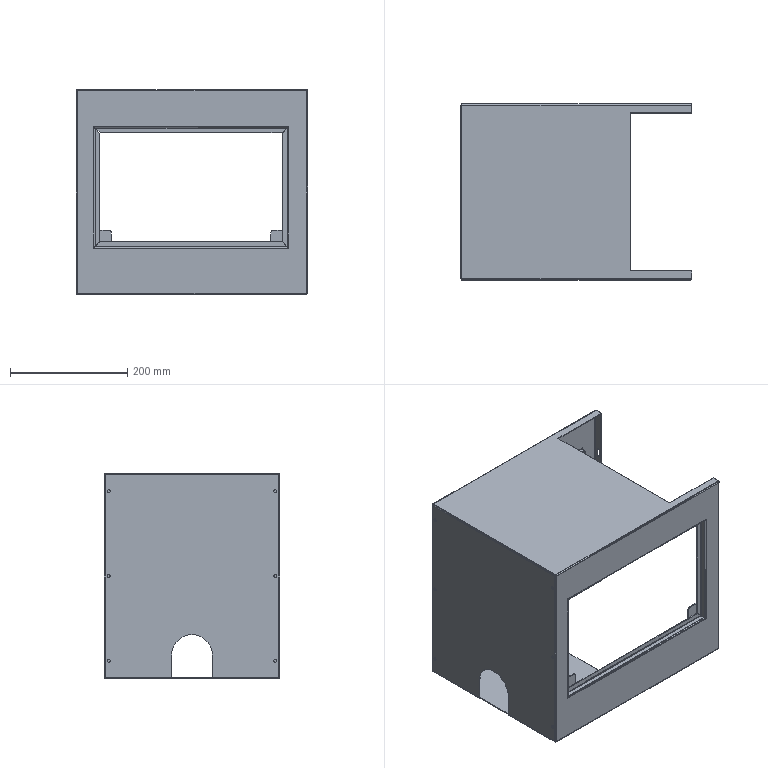Part | SolidWorks | features ICE 5, EdgeFlange 4, Cut 1, Fillet 1, FlatPattern 1, HoleWzd 1, LPattern 1, MirrorPattern 1, SMBaseFlange 1, SheetMetal 1 | 1 solid | 277 faces | box 395 x 300 x 350 mm | volume 661640 mm3 | plane 153 | cylinder 80 | spline 44 | commonest cylinder face diameters 1.473 x25 4.473 x25 5 x12 5.5 x12 10 x4 70 x2